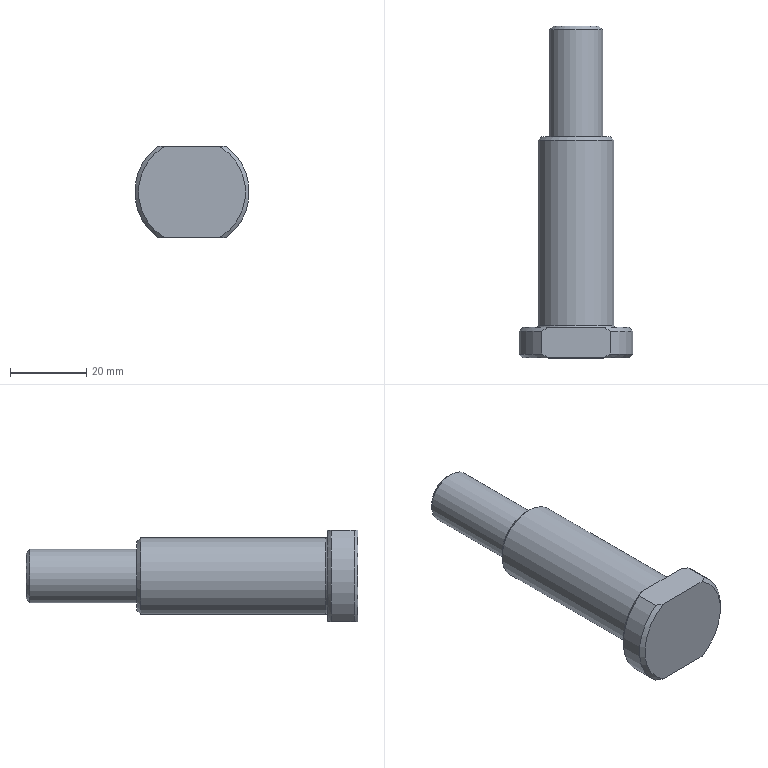Part | STEP file | HL4GZ-1.862.576 (bolt short shaft) | 1 solid | 17 faces | box 30 x 87 x 24 mm | volume 25136 mm3 | cone 6 | plane 6 | cylinder 4 | torus 1 | commonest cylinder face diameters 30 x2 14 x1 20 x1
STEP:
#1=CARTESIAN_POINT('',(0.,0.,0.));
#2=DIRECTION('',(0.,0.,1.));
#3=DIRECTION('',(1.,0.,0.));
#4=AXIS2_PLACEMENT_3D('',#1,#2,#3);
#5=CARTESIAN_POINT('',(1812.33,-148.5,34.265));
#6=VERTEX_POINT('',#5);
#7=CARTESIAN_POINT('',(1810.541,-147.5,34.265));
#8=VERTEX_POINT('',#7);
#9=CARTESIAN_POINT('',(1812.33,-148.5,34.265));
#10=CARTESIAN_POINT('',(1811.723,-148.187,34.265));
#11=CARTESIAN_POINT('',(1811.127,-147.851,34.265));
#12=CARTESIAN_POINT('',(1810.541,-147.5,34.265));
#13=B_SPLINE_CURVE_WITH_KNOTS('',3,(#9,#10,#11,#12),.UNSPECIFIED.,.F.,.F.,(4,4),(0.,1.),.PIECEWISE_BEZIER_KNOTS.);
#14=CARTESIAN_POINT('',(1819.541,-147.5,46.265));
#15=DIRECTION('',(0.,1.,0.));
#16=DIRECTION('',(0.,0.,-1.));
#17=AXIS2_PLACEMENT_3D('',#14,#15,#16);
#18=CONICAL_SURFACE('',#17,15.,0.7854);
#19=CARTESIAN_POINT('',(0.5411,-1.));
#20=CARTESIAN_POINT('',(0.6435,0.));
#21=B_SPLINE_CURVE_WITH_KNOTS('',1,(#19,#20),.UNSPECIFIED.,.F.,.F.,(2,2),(0.,1.),.PIECEWISE_BEZIER_KNOTS.);
#22=(GEOMETRIC_REPRESENTATION_CONTEXT(2)PARAMETRIC_REPRESENTATION_CONTEXT()REPRESENTATION_CONTEXT('',''));
#23=DEFINITIONAL_REPRESENTATION('',(#21),#22);
#24=PCURVE('',#18,#23);
#25=CARTESIAN_POINT('',(1831.291,-151.5,34.265));
#26=DIRECTION('',(0.,0.,1.));
#27=DIRECTION('',(-1.,0.,0.));
#28=AXIS2_PLACEMENT_3D('',#25,#26,#27);
#29=PLANE('',#28);
#30=CARTESIAN_POINT('',(18.961,-3.));
#31=CARTESIAN_POINT('',(19.568,-3.313));
#32=CARTESIAN_POINT('',(20.164,-3.649));
#33=CARTESIAN_POINT('',(20.75,-4.));
#34=B_SPLINE_CURVE_WITH_KNOTS('',3,(#30,#31,#32,#33),.UNSPECIFIED.,.F.,.F.,(4,4),(0.,1.),.PIECEWISE_BEZIER_KNOTS.);
#35=(GEOMETRIC_REPRESENTATION_CONTEXT(2)PARAMETRIC_REPRESENTATION_CONTEXT()REPRESENTATION_CONTEXT('',''));
#36=DEFINITIONAL_REPRESENTATION('',(#34),#35);
#37=PCURVE('',#29,#36);
#38=SURFACE_CURVE('',#13,(#24,#37),.PCURVE_S1.);
#39=EDGE_CURVE('',#6,#8,#38,.T.);
#40=ORIENTED_EDGE('',*,*,#39,.F.);
#41=CARTESIAN_POINT('',(1812.33,-148.5,58.265));
#42=VERTEX_POINT('',#41);
#43=CARTESIAN_POINT('',(1819.541,-148.5,46.265));
#44=DIRECTION('',(0.,-1.,0.));
#45=DIRECTION('',(0.,0.,1.));
#46=AXIS2_PLACEMENT_3D('',#43,#44,#45);
#47=CIRCLE('',#46,14.);
#48=CARTESIAN_POINT('',(3.142,-1.));
#49=DIRECTION('',(-1.,0.));
#50=VECTOR('',#49,1.);
#51=LINE('',#48,#50);
#52=(GEOMETRIC_REPRESENTATION_CONTEXT(2)PARAMETRIC_REPRESENTATION_CONTEXT()REPRESENTATION_CONTEXT('',''));
#53=DEFINITIONAL_REPRESENTATION('',(#51),#52);
#54=PCURVE('',#18,#53);
#55=CARTESIAN_POINT('',(1819.541,-148.5,46.265));
#56=DIRECTION('',(0.,1.,0.));
#57=DIRECTION('',(0.,0.,-1.));
#58=AXIS2_PLACEMENT_3D('',#55,#56,#57);
#59=PLANE('',#58);
#60=CARTESIAN_POINT('',(-14.,0.));
#61=CARTESIAN_POINT('',(-14.,24.249));
#62=CARTESIAN_POINT('',(7.,12.124));
#63=CARTESIAN_POINT('',(28.,0.));
#64=CARTESIAN_POINT('',(7.,-12.124));
#65=CARTESIAN_POINT('',(-14.,-24.249));
#66=CARTESIAN_POINT('',(-14.,0.));
#67=(BOUNDED_CURVE()B_SPLINE_CURVE(2,(#60,#61,#62,#63,#64,#65,#66),.UNSPECIFIED.,.T.,.F.)B_SPLINE_CURVE_WITH_KNOTS((1,2,2,2,2,1),(-2.094,0.,2.094,4.189,6.283,8.378),.UNSPECIFIED.)CURVE()GEOMETRIC_REPRESENTATION_ITEM()RATIONAL_B_SPLINE_CURVE((1.,0.5,1.,0.5,1.,0.5,1.))REPRESENTATION_ITEM(''));
#68=(GEOMETRIC_REPRESENTATION_CONTEXT(2)PARAMETRIC_REPRESENTATION_CONTEXT()REPRESENTATION_CONTEXT('',''));
#69=DEFINITIONAL_REPRESENTATION('',(#67),#68);
#70=PCURVE('',#59,#69);
#71=SURFACE_CURVE('',#47,(#54,#70),.PCURVE_S1.);
#72=EDGE_CURVE('',#42,#6,#71,.T.);
#73=ORIENTED_EDGE('',*,*,#72,.F.);
#74=CARTESIAN_POINT('',(1810.541,-147.5,58.265));
#75=VERTEX_POINT('',#74);
#76=CARTESIAN_POINT('',(1810.541,-147.5,58.265));
#77=CARTESIAN_POINT('',(1811.127,-147.851,58.265));
#78=CARTESIAN_POINT('',(1811.723,-148.187,58.265));
#79=CARTESIAN_POINT('',(1812.33,-148.5,58.265));
#80=B_SPLINE_CURVE_WITH_KNOTS('',3,(#76,#77,#78,#79),.UNSPECIFIED.,.F.,.F.,(4,4),(0.,1.),.PIECEWISE_BEZIER_KNOTS.);
#81=CARTESIAN_POINT('',(2.498,0.));
#82=CARTESIAN_POINT('',(2.6,-1.));
#83=B_SPLINE_CURVE_WITH_KNOTS('',1,(#81,#82),.UNSPECIFIED.,.F.,.F.,(2,2),(0.,1.),.PIECEWISE_BEZIER_KNOTS.);
#84=(GEOMETRIC_REPRESENTATION_CONTEXT(2)PARAMETRIC_REPRESENTATION_CONTEXT()REPRESENTATION_CONTEXT('',''));
#85=DEFINITIONAL_REPRESENTATION('',(#83),#84);
#86=PCURVE('',#18,#85);
#87=CARTESIAN_POINT('',(1835.541,-151.5,58.265));
#88=DIRECTION('',(0.,0.,-1.));
#89=DIRECTION('',(1.,0.,0.));
#90=AXIS2_PLACEMENT_3D('',#87,#88,#89);
#91=PLANE('',#90);
#92=CARTESIAN_POINT('',(-25.,-4.));
#93=CARTESIAN_POINT('',(-24.414,-3.649));
#94=CARTESIAN_POINT('',(-23.818,-3.313));
#95=CARTESIAN_POINT('',(-23.211,-3.));
#96=B_SPLINE_CURVE_WITH_KNOTS('',3,(#92,#93,#94,#95),.UNSPECIFIED.,.F.,.F.,(4,4),(0.,1.),.PIECEWISE_BEZIER_KNOTS.);
#97=(GEOMETRIC_REPRESENTATION_CONTEXT(2)PARAMETRIC_REPRESENTATION_CONTEXT()REPRESENTATION_CONTEXT('',''));
#98=DEFINITIONAL_REPRESENTATION('',(#96),#97);
#99=PCURVE('',#91,#98);
#100=SURFACE_CURVE('',#80,(#86,#99),.PCURVE_S1.);
#101=EDGE_CURVE('',#75,#42,#100,.T.);
#102=ORIENTED_EDGE('',*,*,#101,.F.);
#103=CARTESIAN_POINT('',(1819.541,-147.5,46.265));
#104=DIRECTION('',(0.,1.,0.));
#105=DIRECTION('',(0.,0.,1.));
#106=AXIS2_PLACEMENT_3D('',#103,#104,#105);
#107=CIRCLE('',#106,15.);
#108=CARTESIAN_POINT('',(-3.142,0.));
#109=DIRECTION('',(1.,0.));
#110=VECTOR('',#109,1.);
#111=LINE('',#108,#110);
#112=(GEOMETRIC_REPRESENTATION_CONTEXT(2)PARAMETRIC_REPRESENTATION_CONTEXT()REPRESENTATION_CONTEXT('',''));
#113=DEFINITIONAL_REPRESENTATION('',(#111),#112);
#114=PCURVE('',#18,#113);
#115=CARTESIAN_POINT('',(1819.541,-140.5,46.265));
#116=DIRECTION('',(0.,1.,0.));
#117=DIRECTION('',(0.,0.,-1.));
#118=AXIS2_PLACEMENT_3D('',#115,#116,#117);
#119=CYLINDRICAL_SURFACE('',#118,15.);
#120=CARTESIAN_POINT('',(-3.142,-7.));
#121=DIRECTION('',(1.,0.));
#122=VECTOR('',#121,1.);
#123=LINE('',#120,#122);
#124=(GEOMETRIC_REPRESENTATION_CONTEXT(2)PARAMETRIC_REPRESENTATION_CONTEXT()REPRESENTATION_CONTEXT('',''));
#125=DEFINITIONAL_REPRESENTATION('',(#123),#124);
#126=PCURVE('',#119,#125);
#127=SURFACE_CURVE('',#107,(#114,#126),.PCURVE_S1.);
#128=EDGE_CURVE('',#8,#75,#127,.T.);
#129=ORIENTED_EDGE('',*,*,#128,.F.);
#130=EDGE_LOOP('',(#40,#73,#102,#129));
#131=FACE_BOUND('',#130,.T.);
#132=ADVANCED_FACE('',(#131),#18,.T.);
#133=CARTESIAN_POINT('',(1810.541,-141.5,34.265));
#134=VERTEX_POINT('',#133);
#135=CARTESIAN_POINT('',(1812.33,-140.5,34.265));
#136=VERTEX_POINT('',#135);
#137=CARTESIAN_POINT('',(1810.541,-141.5,34.265));
#138=CARTESIAN_POINT('',(1811.127,-141.148,34.265));
#139=CARTESIAN_POINT('',(1811.723,-140.813,34.265));
#140=CARTESIAN_POINT('',(1812.33,-140.5,34.265));
#141=B_SPLINE_CURVE_WITH_KNOTS('',3,(#137,#138,#139,#140),.UNSPECIFIED.,.F.,.F.,(4,4),(0.,1.),.PIECEWISE_BEZIER_KNOTS.);
#142=CARTESIAN_POINT('',(1819.541,-140.5,46.265));
#143=DIRECTION('',(0.,-1.,0.));
#144=DIRECTION('',(0.,0.,1.));
#145=AXIS2_PLACEMENT_3D('',#142,#143,#144);
#146=CONICAL_SURFACE('',#145,14.,0.7854);
#147=CARTESIAN_POINT('',(2.498,1.));
#148=CARTESIAN_POINT('',(2.6,0.));
#149=B_SPLINE_CURVE_WITH_KNOTS('',1,(#147,#148),.UNSPECIFIED.,.F.,.F.,(2,2),(0.,1.),.PIECEWISE_BEZIER_KNOTS.);
#150=(GEOMETRIC_REPRESENTATION_CONTEXT(2)PARAMETRIC_REPRESENTATION_CONTEXT()REPRESENTATION_CONTEXT('',''));
#151=DEFINITIONAL_REPRESENTATION('',(#149),#150);
#152=PCURVE('',#146,#151);
#153=CARTESIAN_POINT('',(20.75,-10.));
#154=CARTESIAN_POINT('',(20.164,-10.351));
#155=CARTESIAN_POINT('',(19.568,-10.687));
#156=CARTESIAN_POINT('',(18.961,-11.));
#157=B_SPLINE_CURVE_WITH_KNOTS('',3,(#153,#154,#155,#156),.UNSPECIFIED.,.F.,.F.,(4,4),(0.,1.),.PIECEWISE_BEZIER_KNOTS.);
#158=(GEOMETRIC_REPRESENTATION_CONTEXT(2)PARAMETRIC_REPRESENTATION_CONTEXT()REPRESENTATION_CONTEXT('',''));
#159=DEFINITIONAL_REPRESENTATION('',(#157),#158);
#160=PCURVE('',#29,#159);
#161=SURFACE_CURVE('',#141,(#152,#160),.PCURVE_S1.);
#162=EDGE_CURVE('',#134,#136,#161,.T.);
#163=ORIENTED_EDGE('',*,*,#162,.F.);
#164=CARTESIAN_POINT('',(1810.541,-141.5,58.265));
#165=VERTEX_POINT('',#164);
#166=CARTESIAN_POINT('',(1819.541,-141.5,46.265));
#167=DIRECTION('',(0.,-1.,0.));
#168=DIRECTION('',(0.,0.,1.));
#169=AXIS2_PLACEMENT_3D('',#166,#167,#168);
#170=CIRCLE('',#169,15.);
#171=CARTESIAN_POINT('',(0.,1.));
#172=DIRECTION('',(1.,0.));
#173=VECTOR('',#172,1.);
#174=LINE('',#171,#173);
#175=(GEOMETRIC_REPRESENTATION_CONTEXT(2)PARAMETRIC_REPRESENTATION_CONTEXT()REPRESENTATION_CONTEXT('',''));
#176=DEFINITIONAL_REPRESENTATION('',(#174),#175);
#177=PCURVE('',#146,#176);
#178=CARTESIAN_POINT('',(3.142,-1.));
#179=DIRECTION('',(-1.,0.));
#180=VECTOR('',#179,1.);
#181=LINE('',#178,#180);
#182=(GEOMETRIC_REPRESENTATION_CONTEXT(2)PARAMETRIC_REPRESENTATION_CONTEXT()REPRESENTATION_CONTEXT('',''));
#183=DEFINITIONAL_REPRESENTATION('',(#181),#182);
#184=PCURVE('',#119,#183);
#185=SURFACE_CURVE('',#170,(#177,#184),.PCURVE_S1.);
#186=EDGE_CURVE('',#165,#134,#185,.T.);
#187=ORIENTED_EDGE('',*,*,#186,.F.);
#188=CARTESIAN_POINT('',(1812.33,-140.5,58.265));
#189=VERTEX_POINT('',#188);
#190=CARTESIAN_POINT('',(1812.33,-140.5,58.265));
#191=CARTESIAN_POINT('',(1811.723,-140.813,58.265));
#192=CARTESIAN_POINT('',(1811.127,-141.148,58.265));
#193=CARTESIAN_POINT('',(1810.541,-141.5,58.265));
#194=B_SPLINE_CURVE_WITH_KNOTS('',3,(#190,#191,#192,#193),.UNSPECIFIED.,.F.,.F.,(4,4),(0.,1.),.PIECEWISE_BEZIER_KNOTS.);
#195=CARTESIAN_POINT('',(0.5411,0.));
#196=CARTESIAN_POINT('',(0.6435,1.));
#197=B_SPLINE_CURVE_WITH_KNOTS('',1,(#195,#196),.UNSPECIFIED.,.F.,.F.,(2,2),(0.,1.),.PIECEWISE_BEZIER_KNOTS.);
#198=(GEOMETRIC_REPRESENTATION_CONTEXT(2)PARAMETRIC_REPRESENTATION_CONTEXT()REPRESENTATION_CONTEXT('',''));
#199=DEFINITIONAL_REPRESENTATION('',(#197),#198);
#200=PCURVE('',#146,#199);
#201=CARTESIAN_POINT('',(-23.211,-11.));
#202=CARTESIAN_POINT('',(-23.818,-10.687));
#203=CARTESIAN_POINT('',(-24.414,-10.351));
#204=CARTESIAN_POINT('',(-25.,-10.));
#205=B_SPLINE_CURVE_WITH_KNOTS('',3,(#201,#202,#203,#204),.UNSPECIFIED.,.F.,.F.,(4,4),(0.,1.),.PIECEWISE_BEZIER_KNOTS.);
#206=(GEOMETRIC_REPRESENTATION_CONTEXT(2)PARAMETRIC_REPRESENTATION_CONTEXT()REPRESENTATION_CONTEXT('',''));
#207=DEFINITIONAL_REPRESENTATION('',(#205),#206);
#208=PCURVE('',#91,#207);
#209=SURFACE_CURVE('',#194,(#200,#208),.PCURVE_S1.);
#210=EDGE_CURVE('',#189,#165,#209,.T.);
#211=ORIENTED_EDGE('',*,*,#210,.F.);
#212=CARTESIAN_POINT('',(1819.541,-140.5,46.265));
#213=DIRECTION('',(0.,1.,0.));
#214=DIRECTION('',(0.,0.,1.));
#215=AXIS2_PLACEMENT_3D('',#212,#213,#214);
#216=CIRCLE('',#215,14.);
#217=CARTESIAN_POINT('',(6.283,0.));
#218=DIRECTION('',(-1.,0.));
#219=VECTOR('',#218,1.);
#220=LINE('',#217,#219);
#221=(GEOMETRIC_REPRESENTATION_CONTEXT(2)PARAMETRIC_REPRESENTATION_CONTEXT()REPRESENTATION_CONTEXT('',''));
#222=DEFINITIONAL_REPRESENTATION('',(#220),#221);
#223=PCURVE('',#146,#222);
#224=CARTESIAN_POINT('',(1804.541,-140.5,46.265));
#225=DIRECTION('',(0.,1.,0.));
#226=DIRECTION('',(0.,0.,-1.));
#227=AXIS2_PLACEMENT_3D('',#224,#225,#226);
#228=PLANE('',#227);
#229=CARTESIAN_POINT('',(0.,-15.));
#230=DIRECTION('',(-1.,0.));
#231=AXIS2_PLACEMENT_2D('',#229,#230);
#232=CIRCLE('',#231,14.);
#233=(GEOMETRIC_REPRESENTATION_CONTEXT(2)PARAMETRIC_REPRESENTATION_CONTEXT()REPRESENTATION_CONTEXT('',''));
#234=DEFINITIONAL_REPRESENTATION('',(#232),#233);
#235=PCURVE('',#228,#234);
#236=SURFACE_CURVE('',#216,(#223,#235),.PCURVE_S1.);
#237=EDGE_CURVE('',#136,#189,#236,.T.);
#238=ORIENTED_EDGE('',*,*,#237,.F.);
#239=EDGE_LOOP('',(#163,#187,#211,#238));
#240=FACE_BOUND('',#239,.T.);
#241=ADVANCED_FACE('',(#240),#146,.T.);
#242=CARTESIAN_POINT('',(1828.541,-141.5,58.265));
#243=VERTEX_POINT('',#242);
#244=CARTESIAN_POINT('',(1826.752,-140.5,58.265));
#245=VERTEX_POINT('',#244);
#246=CARTESIAN_POINT('',(1828.541,-141.5,58.265));
#247=CARTESIAN_POINT('',(1827.955,-141.148,58.265));
#248=CARTESIAN_POINT('',(1827.36,-140.813,58.265));
#249=CARTESIAN_POINT('',(1826.752,-140.5,58.265));
#250=B_SPLINE_CURVE_WITH_KNOTS('',3,(#246,#247,#248,#249),.UNSPECIFIED.,.F.,.F.,(4,4),(0.,1.),.PIECEWISE_BEZIER_KNOTS.);
#251=CARTESIAN_POINT('',(1819.541,-140.5,46.265));
#252=DIRECTION('',(0.,-1.,0.));
#253=DIRECTION('',(0.,0.,1.));
#254=AXIS2_PLACEMENT_3D('',#251,#252,#253);
#255=CONICAL_SURFACE('',#254,14.,0.7854);
#256=CARTESIAN_POINT('',(5.64,1.));
#257=CARTESIAN_POINT('',(5.742,0.));
#258=B_SPLINE_CURVE_WITH_KNOTS('',1,(#256,#257),.UNSPECIFIED.,.F.,.F.,(2,2),(0.,1.),.PIECEWISE_BEZIER_KNOTS.);
#259=(GEOMETRIC_REPRESENTATION_CONTEXT(2)PARAMETRIC_REPRESENTATION_CONTEXT()REPRESENTATION_CONTEXT('',''));
#260=DEFINITIONAL_REPRESENTATION('',(#258),#259);
#261=PCURVE('',#255,#260);
#262=CARTESIAN_POINT('',(-7.,-10.));
#263=CARTESIAN_POINT('',(-7.586,-10.351));
#264=CARTESIAN_POINT('',(-8.182,-10.687));
#265=CARTESIAN_POINT('',(-8.789,-11.));
#266=B_SPLINE_CURVE_WITH_KNOTS('',3,(#262,#263,#264,#265),.UNSPECIFIED.,.F.,.F.,(4,4),(0.,1.),.PIECEWISE_BEZIER_KNOTS.);
#267=(GEOMETRIC_REPRESENTATION_CONTEXT(2)PARAMETRIC_REPRESENTATION_CONTEXT()REPRESENTATION_CONTEXT('',''));
#268=DEFINITIONAL_REPRESENTATION('',(#266),#267);
#269=PCURVE('',#91,#268);
#270=SURFACE_CURVE('',#250,(#261,#269),.PCURVE_S1.);
#271=EDGE_CURVE('',#243,#245,#270,.T.);
#272=ORIENTED_EDGE('',*,*,#271,.F.);
#273=CARTESIAN_POINT('',(1828.541,-141.5,34.265));
#274=VERTEX_POINT('',#273);
#275=CARTESIAN_POINT('',(1819.541,-141.5,46.265));
#276=DIRECTION('',(0.,-1.,0.));
#277=DIRECTION('',(0.,0.,1.));
#278=AXIS2_PLACEMENT_3D('',#275,#276,#277);
#279=CIRCLE('',#278,15.);
#280=CARTESIAN_POINT('',(0.,1.));
#281=DIRECTION('',(1.,0.));
#282=VECTOR('',#281,1.);
#283=LINE('',#280,#282);
#284=(GEOMETRIC_REPRESENTATION_CONTEXT(2)PARAMETRIC_REPRESENTATION_CONTEXT()REPRESENTATION_CONTEXT('',''));
#285=DEFINITIONAL_REPRESENTATION('',(#283),#284);
#286=PCURVE('',#255,#285);
#287=CARTESIAN_POINT('',(1819.541,-140.5,46.265));
#288=DIRECTION('',(0.,1.,0.));
#289=DIRECTION('',(0.,0.,-1.));
#290=AXIS2_PLACEMENT_3D('',#287,#288,#289);
#291=CYLINDRICAL_SURFACE('',#290,15.);
#292=CARTESIAN_POINT('',(9.425,-1.));
#293=DIRECTION('',(-1.,0.));
#294=VECTOR('',#293,1.);
#295=LINE('',#292,#294);
#296=(GEOMETRIC_REPRESENTATION_CONTEXT(2)PARAMETRIC_REPRESENTATION_CONTEXT()REPRESENTATION_CONTEXT('',''));
#297=DEFINITIONAL_REPRESENTATION('',(#295),#296);
#298=PCURVE('',#291,#297);
#299=SURFACE_CURVE('',#279,(#286,#298),.PCURVE_S1.);
#300=EDGE_CURVE('',#274,#243,#299,.T.);
#301=ORIENTED_EDGE('',*,*,#300,.F.);
#302=CARTESIAN_POINT('',(1826.752,-140.5,34.265));
#303=VERTEX_POINT('',#302);
#304=CARTESIAN_POINT('',(1826.752,-140.5,34.265));
#305=CARTESIAN_POINT('',(1827.36,-140.813,34.265));
#306=CARTESIAN_POINT('',(1827.955,-141.148,34.265));
#307=CARTESIAN_POINT('',(1828.541,-141.5,34.265));
#308=B_SPLINE_CURVE_WITH_KNOTS('',3,(#304,#305,#306,#307),.UNSPECIFIED.,.F.,.F.,(4,4),(0.,1.),.PIECEWISE_BEZIER_KNOTS.);
#309=CARTESIAN_POINT('',(3.683,0.));
#310=CARTESIAN_POINT('',(3.785,1.));
#311=B_SPLINE_CURVE_WITH_KNOTS('',1,(#309,#310),.UNSPECIFIED.,.F.,.F.,(2,2),(0.,1.),.PIECEWISE_BEZIER_KNOTS.);
#312=(GEOMETRIC_REPRESENTATION_CONTEXT(2)PARAMETRIC_REPRESENTATION_CONTEXT()REPRESENTATION_CONTEXT('',''));
#313=DEFINITIONAL_REPRESENTATION('',(#311),#312);
#314=PCURVE('',#255,#313);
#315=CARTESIAN_POINT('',(4.539,-11.));
#316=CARTESIAN_POINT('',(3.932,-10.687));
#317=CARTESIAN_POINT('',(3.336,-10.351));
#318=CARTESIAN_POINT('',(2.75,-10.));
#319=B_SPLINE_CURVE_WITH_KNOTS('',3,(#315,#316,#317,#318),.UNSPECIFIED.,.F.,.F.,(4,4),(0.,1.),.PIECEWISE_BEZIER_KNOTS.);
#320=(GEOMETRIC_REPRESENTATION_CONTEXT(2)PARAMETRIC_REPRESENTATION_CONTEXT()REPRESENTATION_CONTEXT('',''));
#321=DEFINITIONAL_REPRESENTATION('',(#319),#320);
#322=PCURVE('',#29,#321);
#323=SURFACE_CURVE('',#308,(#314,#322),.PCURVE_S1.);
#324=EDGE_CURVE('',#303,#274,#323,.T.);
#325=ORIENTED_EDGE('',*,*,#324,.F.);
#326=CARTESIAN_POINT('',(1819.541,-140.5,46.265));
#327=DIRECTION('',(0.,1.,0.));
#328=DIRECTION('',(0.,0.,1.));
#329=AXIS2_PLACEMENT_3D('',#326,#327,#328);
#330=CIRCLE('',#329,14.);
#331=CARTESIAN_POINT('',(6.283,0.));
#332=DIRECTION('',(-1.,0.));
#333=VECTOR('',#332,1.);
#334=LINE('',#331,#333);
#335=(GEOMETRIC_REPRESENTATION_CONTEXT(2)PARAMETRIC_REPRESENTATION_CONTEXT()REPRESENTATION_CONTEXT('',''));
#336=DEFINITIONAL_REPRESENTATION('',(#334),#335);
#337=PCURVE('',#255,#336);
#338=CARTESIAN_POINT('',(0.,-15.));
#339=DIRECTION('',(-1.,0.));
#340=AXIS2_PLACEMENT_2D('',#338,#339);
#341=CIRCLE('',#340,14.);
#342=(GEOMETRIC_REPRESENTATION_CONTEXT(2)PARAMETRIC_REPRESENTATION_CONTEXT()REPRESENTATION_CONTEXT('',''));
#343=DEFINITIONAL_REPRESENTATION('',(#341),#342);
#344=PCURVE('',#228,#343);
#345=SURFACE_CURVE('',#330,(#337,#344),.PCURVE_S1.);
#346=EDGE_CURVE('',#245,#303,#345,.T.);
#347=ORIENTED_EDGE('',*,*,#346,.F.);
#348=EDGE_LOOP('',(#272,#301,#325,#347));
#349=FACE_BOUND('',#348,.T.);
#350=ADVANCED_FACE('',(#349),#255,.T.);
#351=CARTESIAN_POINT('',(1826.752,-148.5,58.265));
#352=VERTEX_POINT('',#351);
#353=CARTESIAN_POINT('',(1828.541,-147.5,58.265));
#354=VERTEX_POINT('',#353);
#355=CARTESIAN_POINT('',(1826.752,-148.5,58.265));
#356=CARTESIAN_POINT('',(1827.36,-148.187,58.265));
#357=CARTESIAN_POINT('',(1827.955,-147.851,58.265));
#358=CARTESIAN_POINT('',(1828.541,-147.5,58.265));
#359=B_SPLINE_CURVE_WITH_KNOTS('',3,(#355,#356,#357,#358),.UNSPECIFIED.,.F.,.F.,(4,4),(0.,1.),.PIECEWISE_BEZIER_KNOTS.);
#360=CARTESIAN_POINT('',(1819.541,-147.5,46.265));
#361=DIRECTION('',(0.,1.,0.));
#362=DIRECTION('',(0.,0.,-1.));
#363=AXIS2_PLACEMENT_3D('',#360,#361,#362);
#364=CONICAL_SURFACE('',#363,15.,0.7854);
#365=CARTESIAN_POINT('',(3.683,-1.));
#366=CARTESIAN_POINT('',(3.785,0.));
#367=B_SPLINE_CURVE_WITH_KNOTS('',1,(#365,#366),.UNSPECIFIED.,.F.,.F.,(2,2),(0.,1.),.PIECEWISE_BEZIER_KNOTS.);
#368=(GEOMETRIC_REPRESENTATION_CONTEXT(2)PARAMETRIC_REPRESENTATION_CONTEXT()REPRESENTATION_CONTEXT('',''));
#369=DEFINITIONAL_REPRESENTATION('',(#367),#368);
#370=PCURVE('',#364,#369);
#371=CARTESIAN_POINT('',(-8.789,-3.));
#372=CARTESIAN_POINT('',(-8.182,-3.313));
#373=CARTESIAN_POINT('',(-7.586,-3.649));
#374=CARTESIAN_POINT('',(-7.,-4.));
#375=B_SPLINE_CURVE_WITH_KNOTS('',3,(#371,#372,#373,#374),.UNSPECIFIED.,.F.,.F.,(4,4),(0.,1.),.PIECEWISE_BEZIER_KNOTS.);
#376=(GEOMETRIC_REPRESENTATION_CONTEXT(2)PARAMETRIC_REPRESENTATION_CONTEXT()REPRESENTATION_CONTEXT('',''));
#377=DEFINITIONAL_REPRESENTATION('',(#375),#376);
#378=PCURVE('',#91,#377);
#379=SURFACE_CURVE('',#359,(#370,#378),.PCURVE_S1.);
#380=EDGE_CURVE('',#352,#354,#379,.T.);
#381=ORIENTED_EDGE('',*,*,#380,.F.);
#382=CARTESIAN_POINT('',(1826.752,-148.5,34.265));
#383=VERTEX_POINT('',#382);
#384=CARTESIAN_POINT('',(1819.541,-148.5,46.265));
#385=DIRECTION('',(0.,-1.,0.));
#386=DIRECTION('',(0.,0.,1.));
#387=AXIS2_PLACEMENT_3D('',#384,#385,#386);
#388=CIRCLE('',#387,14.);
#389=CARTESIAN_POINT('',(9.425,-1.));
#390=DIRECTION('',(-1.,0.));
#391=VECTOR('',#390,1.);
#392=LINE('',#389,#391);
#393=(GEOMETRIC_REPRESENTATION_CONTEXT(2)PARAMETRIC_REPRESENTATION_CONTEXT()REPRESENTATION_CONTEXT('',''));
#394=DEFINITIONAL_REPRESENTATION('',(#392),#393);
#395=PCURVE('',#364,#394);
#396=CARTESIAN_POINT('',(-14.,0.));
#397=CARTESIAN_POINT('',(-14.,24.249));
#398=CARTESIAN_POINT('',(7.,12.124));
#399=CARTESIAN_POINT('',(28.,0.));
#400=CARTESIAN_POINT('',(7.,-12.124));
#401=CARTESIAN_POINT('',(-14.,-24.249));
#402=CARTESIAN_POINT('',(-14.,0.));
#403=(BOUNDED_CURVE()B_SPLINE_CURVE(2,(#396,#397,#398,#399,#400,#401,#402),.UNSPECIFIED.,.T.,.F.)B_SPLINE_CURVE_WITH_KNOTS((1,2,2,2,2,1),(-2.094,0.,2.094,4.189,6.283,8.378),.UNSPECIFIED.)CURVE()GEOMETRIC_REPRESENTATION_ITEM()RATIONAL_B_SPLINE_CURVE((1.,0.5,1.,0.5,1.,0.5,1.))REPRESENTATION_ITEM(''));
#404=(GEOMETRIC_REPRESENTATION_CONTEXT(2)PARAMETRIC_REPRESENTATION_CONTEXT()REPRESENTATION_CONTEXT('',''));
#405=DEFINITIONAL_REPRESENTATION('',(#403),#404);
#406=PCURVE('',#59,#405);
#407=SURFACE_CURVE('',#388,(#395,#406),.PCURVE_S1.);
#408=EDGE_CURVE('',#383,#352,#407,.T.);
#409=ORIENTED_EDGE('',*,*,#408,.F.);
#410=CARTESIAN_POINT('',(1828.541,-147.5,34.265));
#411=VERTEX_POINT('',#410);
#412=CARTESIAN_POINT('',(1828.541,-147.5,34.265));
#413=CARTESIAN_POINT('',(1827.955,-147.851,34.265));
#414=CARTESIAN_POINT('',(1827.36,-148.187,34.265));
#415=CARTESIAN_POINT('',(1826.752,-148.5,34.265));
#416=B_SPLINE_CURVE_WITH_KNOTS('',3,(#412,#413,#414,#415),.UNSPECIFIED.,.F.,.F.,(4,4),(0.,1.),.PIECEWISE_BEZIER_KNOTS.);
#417=CARTESIAN_POINT('',(5.64,0.));
#418=CARTESIAN_POINT('',(5.742,-1.));
#419=B_SPLINE_CURVE_WITH_KNOTS('',1,(#417,#418),.UNSPECIFIED.,.F.,.F.,(2,2),(0.,1.),.PIECEWISE_BEZIER_KNOTS.);
#420=(GEOMETRIC_REPRESENTATION_CONTEXT(2)PARAMETRIC_REPRESENTATION_CONTEXT()REPRESENTATION_CONTEXT('',''));
#421=DEFINITIONAL_REPRESENTATION('',(#419),#420);
#422=PCURVE('',#364,#421);
#423=CARTESIAN_POINT('',(2.75,-4.));
#424=CARTESIAN_POINT('',(3.336,-3.649));
#425=CARTESIAN_POINT('',(3.932,-3.313));
#426=CARTESIAN_POINT('',(4.539,-3.));
#427=B_SPLINE_CURVE_WITH_KNOTS('',3,(#423,#424,#425,#426),.UNSPECIFIED.,.F.,.F.,(4,4),(0.,1.),.PIECEWISE_BEZIER_KNOTS.);
#428=(GEOMETRIC_REPRESENTATION_CONTEXT(2)PARAMETRIC_REPRESENTATION_CONTEXT()REPRESENTATION_CONTEXT('',''));
#429=DEFINITIONAL_REPRESENTATION('',(#427),#428);
#430=PCURVE('',#29,#429);
#431=SURFACE_CURVE('',#416,(#422,#430),.PCURVE_S1.);
#432=EDGE_CURVE('',#411,#383,#431,.T.);
#433=ORIENTED_EDGE('',*,*,#432,.F.);
#434=CARTESIAN_POINT('',(1819.541,-147.5,46.265));
#435=DIRECTION('',(0.,1.,0.));
#436=DIRECTION('',(0.,0.,1.));
#437=AXIS2_PLACEMENT_3D('',#434,#435,#436);
#438=CIRCLE('',#437,15.);
#439=CARTESIAN_POINT('',(3.142,0.));
#440=DIRECTION('',(1.,0.));
#441=VECTOR('',#440,1.);
#442=LINE('',#439,#441);
#443=(GEOMETRIC_REPRESENTATION_CONTEXT(2)PARAMETRIC_REPRESENTATION_CONTEXT()REPRESENTATION_CONTEXT('',''));
#444=DEFINITIONAL_REPRESENTATION('',(#442),#443);
#445=PCURVE('',#364,#444);
#446=CARTESIAN_POINT('',(3.142,-7.));
#447=DIRECTION('',(1.,0.));
#448=VECTOR('',#447,1.);
#449=LINE('',#446,#448);
#450=(GEOMETRIC_REPRESENTATION_CONTEXT(2)PARAMETRIC_REPRESENTATION_CONTEXT()REPRESENTATION_CONTEXT('',''));
#451=DEFINITIONAL_REPRESENTATION('',(#449),#450);
#452=PCURVE('',#291,#451);
#453=SURFACE_CURVE('',#438,(#445,#452),.PCURVE_S1.);
#454=EDGE_CURVE('',#354,#411,#453,.T.);
#455=ORIENTED_EDGE('',*,*,#454,.F.);
#456=EDGE_LOOP('',(#381,#409,#433,#455));
#457=FACE_BOUND('',#456,.T.);
#458=ADVANCED_FACE('',(#457),#364,.T.);
#459=CARTESIAN_POINT('',(1819.541,-91.5,56.265));
#460=VERTEX_POINT('',#459);
#461=CARTESIAN_POINT('',(1819.541,-91.5,46.265));
#462=DIRECTION('',(0.,-1.,0.));
#463=DIRECTION('',(0.,0.,1.));
#464=AXIS2_PLACEMENT_3D('',#461,#462,#463);
#465=CIRCLE('',#464,10.);
#466=CARTESIAN_POINT('',(1819.541,-91.5,46.265));
#467=DIRECTION('',(0.,-1.,0.));
#468=DIRECTION('',(0.,0.,1.));
#469=AXIS2_PLACEMENT_3D('',#466,#467,#468);
#470=CONICAL_SURFACE('',#469,10.,0.7854);
#471=CARTESIAN_POINT('',(0.,0.));
#472=DIRECTION('',(1.,0.));
#473=VECTOR('',#472,1.);
#474=LINE('',#471,#473);
#475=(GEOMETRIC_REPRESENTATION_CONTEXT(2)PARAMETRIC_REPRESENTATION_CONTEXT()REPRESENTATION_CONTEXT('',''));
#476=DEFINITIONAL_REPRESENTATION('',(#474),#475);
#477=PCURVE('',#470,#476);
#478=CARTESIAN_POINT('',(1819.541,-140.5,46.265));
#479=DIRECTION('',(0.,1.,0.));
#480=DIRECTION('',(0.,0.,-1.));
#481=AXIS2_PLACEMENT_3D('',#478,#479,#480);
#482=CYLINDRICAL_SURFACE('',#481,10.);
#483=CARTESIAN_POINT('',(9.425,49.));
#484=DIRECTION('',(-1.,0.));
#485=VECTOR('',#484,1.);
#486=LINE('',#483,#485);
#487=(GEOMETRIC_REPRESENTATION_CONTEXT(2)PARAMETRIC_REPRESENTATION_CONTEXT()REPRESENTATION_CONTEXT('',''));
#488=DEFINITIONAL_REPRESENTATION('',(#486),#487);
#489=PCURVE('',#482,#488);
#490=SURFACE_CURVE('',#465,(#477,#489),.PCURVE_S1.);
#491=EDGE_CURVE('',#460,#460,#490,.T.);
#492=ORIENTED_EDGE('',*,*,#491,.F.);
#493=CARTESIAN_POINT('',(1819.541,-90.5,55.265));
#494=VERTEX_POINT('',#493);
#495=CARTESIAN_POINT('',(1819.541,-90.5,55.265));
#496=CARTESIAN_POINT('',(1819.541,-91.5,56.265));
#497=B_SPLINE_CURVE_WITH_KNOTS('',1,(#495,#496),.UNSPECIFIED.,.F.,.F.,(2,2),(-1.414,0.),.PIECEWISE_BEZIER_KNOTS.);
#498=CARTESIAN_POINT('',(0.,0.));
#499=DIRECTION('',(0.,1.));
#500=VECTOR('',#499,1.);
#501=LINE('',#498,#500);
#502=(GEOMETRIC_REPRESENTATION_CONTEXT(2)PARAMETRIC_REPRESENTATION_CONTEXT()REPRESENTATION_CONTEXT('',''));
#503=DEFINITIONAL_REPRESENTATION('',(#501),#502);
#504=PCURVE('',#470,#503);
#505=CARTESIAN_POINT('',(6.283,0.));
#506=DIRECTION('',(0.,1.));
#507=VECTOR('',#506,1.);
#508=LINE('',#505,#507);
#509=(GEOMETRIC_REPRESENTATION_CONTEXT(2)PARAMETRIC_REPRESENTATION_CONTEXT()REPRESENTATION_CONTEXT('',''));
#510=DEFINITIONAL_REPRESENTATION('',(#508),#509);
#511=PCURVE('',#470,#510);
#512=SEAM_CURVE('',#497,(#504,#511),.PCURVE_S1.);
#513=EDGE_CURVE('',#494,#460,#512,.T.);
#514=ORIENTED_EDGE('',*,*,#513,.F.);
#515=CARTESIAN_POINT('',(1819.541,-90.5,46.265));
#516=DIRECTION('',(0.,1.,0.));
#517=DIRECTION('',(0.,0.,1.));
#518=AXIS2_PLACEMENT_3D('',#515,#516,#517);
#519=CIRCLE('',#518,9.);
#520=CARTESIAN_POINT('',(6.283,-1.));
#521=DIRECTION('',(-1.,0.));
#522=VECTOR('',#521,1.);
#523=LINE('',#520,#522);
#524=(GEOMETRIC_REPRESENTATION_CONTEXT(2)PARAMETRIC_REPRESENTATION_CONTEXT()REPRESENTATION_CONTEXT('',''));
#525=DEFINITIONAL_REPRESENTATION('',(#523),#524);
#526=PCURVE('',#470,#525);
#527=CARTESIAN_POINT('',(1809.541,-90.5,46.265));
#528=DIRECTION('',(0.,1.,0.));
#529=DIRECTION('',(0.,0.,-1.));
#530=AXIS2_PLACEMENT_3D('',#527,#528,#529);
#531=PLANE('',#530);
#532=CARTESIAN_POINT('',(0.,-10.));
#533=DIRECTION('',(-1.,0.));
#534=AXIS2_PLACEMENT_2D('',#532,#533);
#535=CIRCLE('',#534,9.);
#536=(GEOMETRIC_REPRESENTATION_CONTEXT(2)PARAMETRIC_REPRESENTATION_CONTEXT()REPRESENTATION_CONTEXT('',''));
#537=DEFINITIONAL_REPRESENTATION('',(#535),#536);
#538=PCURVE('',#531,#537);
#539=SURFACE_CURVE('',#519,(#526,#538),.PCURVE_S1.);
#540=EDGE_CURVE('',#494,#494,#539,.T.);
#541=ORIENTED_EDGE('',*,*,#540,.F.);
#542=ORIENTED_EDGE('',*,*,#513,.T.);
#543=EDGE_LOOP('',(#492,#514,#541,#542));
#544=FACE_BOUND('',#543,.T.);
#545=ADVANCED_FACE('',(#544),#470,.T.);
#546=CARTESIAN_POINT('',(1819.541,-140.,56.265));
#547=VERTEX_POINT('',#546);
#548=CARTESIAN_POINT('',(1819.541,-140.,46.265));
#549=DIRECTION('',(0.,1.,0.));
#550=DIRECTION('',(0.,0.,1.));
#551=AXIS2_PLACEMENT_3D('',#548,#549,#550);
#552=CIRCLE('',#551,10.);
#553=CARTESIAN_POINT('',(1819.541,-140.,46.265));
#554=DIRECTION('',(0.,1.,0.));
#555=DIRECTION('',(0.,0.,-1.));
#556=AXIS2_PLACEMENT_3D('',#553,#554,#555);
#557=TOROIDAL_SURFACE('',#556,10.5,0.5);
#558=CARTESIAN_POINT('',(3.142,3.142));
#559=DIRECTION('',(1.,0.));
#560=VECTOR('',#559,1.);
#561=LINE('',#558,#560);
#562=(GEOMETRIC_REPRESENTATION_CONTEXT(2)PARAMETRIC_REPRESENTATION_CONTEXT()REPRESENTATION_CONTEXT('',''));
#563=DEFINITIONAL_REPRESENTATION('',(#561),#562);
#564=PCURVE('',#557,#563);
#565=CARTESIAN_POINT('',(3.142,0.5));
#566=DIRECTION('',(1.,0.));
#567=VECTOR('',#566,1.);
#568=LINE('',#565,#567);
#569=(GEOMETRIC_REPRESENTATION_CONTEXT(2)PARAMETRIC_REPRESENTATION_CONTEXT()REPRESENTATION_CONTEXT('',''));
#570=DEFINITIONAL_REPRESENTATION('',(#568),#569);
#571=PCURVE('',#482,#570);
#572=SURFACE_CURVE('',#552,(#564,#571),.PCURVE_S1.);
#573=EDGE_CURVE('',#547,#547,#572,.T.);
#574=ORIENTED_EDGE('',*,*,#573,.T.);
#575=CARTESIAN_POINT('',(1819.541,-140.5,56.765));
#576=VERTEX_POINT('',#575);
#577=CARTESIAN_POINT('',(1819.541,-140.,56.265));
#578=CARTESIAN_POINT('',(1819.541,-140.134,56.265));
#579=CARTESIAN_POINT('',(1819.541,-140.264,56.307));
#580=CARTESIAN_POINT('',(1819.541,-140.376,56.389));
#581=CARTESIAN_POINT('',(1819.541,-140.457,56.501));
#582=CARTESIAN_POINT('',(1819.541,-140.5,56.631));
#583=CARTESIAN_POINT('',(1819.541,-140.5,56.765));
#584=(BOUNDED_CURVE()B_SPLINE_CURVE(6,(#577,#578,#579,#580,#581,#582,#583),.UNSPECIFIED.,.F.,.F.)B_SPLINE_CURVE_WITH_KNOTS((7,7),(3.142,4.712),.PIECEWISE_BEZIER_KNOTS.)CURVE()GEOMETRIC_REPRESENTATION_ITEM()RATIONAL_B_SPLINE_CURVE((1.031,1.01,0.9979,0.994,0.9979,1.01,1.031))REPRESENTATION_ITEM(''));
#585=CARTESIAN_POINT('',(9.425,0.));
#586=DIRECTION('',(0.,1.));
#587=VECTOR('',#586,1.);
#588=LINE('',#585,#587);
#589=(GEOMETRIC_REPRESENTATION_CONTEXT(2)PARAMETRIC_REPRESENTATION_CONTEXT()REPRESENTATION_CONTEXT('',''));
#590=DEFINITIONAL_REPRESENTATION('',(#588),#589);
#591=PCURVE('',#557,#590);
#592=CARTESIAN_POINT('',(3.142,0.));
#593=DIRECTION('',(0.,1.));
#594=VECTOR('',#593,1.);
#595=LINE('',#592,#594);
#596=(GEOMETRIC_REPRESENTATION_CONTEXT(2)PARAMETRIC_REPRESENTATION_CONTEXT()REPRESENTATION_CONTEXT('',''));
#597=DEFINITIONAL_REPRESENTATION('',(#595),#596);
#598=PCURVE('',#557,#597);
#599=SEAM_CURVE('',#584,(#591,#598),.PCURVE_S1.);
#600=EDGE_CURVE('',#547,#576,#599,.T.);
#601=ORIENTED_EDGE('',*,*,#600,.T.);
#602=CARTESIAN_POINT('',(1819.541,-140.5,46.265));
#603=DIRECTION('',(0.,-1.,0.));
#604=DIRECTION('',(0.,0.,1.));
#605=AXIS2_PLACEMENT_3D('',#602,#603,#604);
#606=CIRCLE('',#605,10.5);
#607=CARTESIAN_POINT('',(9.425,4.712));
#608=DIRECTION('',(-1.,0.));
#609=VECTOR('',#608,1.);
#610=LINE('',#607,#609);
#611=(GEOMETRIC_REPRESENTATION_CONTEXT(2)PARAMETRIC_REPRESENTATION_CONTEXT()REPRESENTATION_CONTEXT('',''));
#612=DEFINITIONAL_REPRESENTATION('',(#610),#611);
#613=PCURVE('',#557,#612);
#614=CARTESIAN_POINT('',(-10.5,-15.));
#615=CARTESIAN_POINT('',(-10.5,3.187));
#616=CARTESIAN_POINT('',(5.25,-5.907));
#617=CARTESIAN_POINT('',(21.,-15.));
#618=CARTESIAN_POINT('',(5.25,-24.093));
#619=CARTESIAN_POINT('',(-10.5,-33.187));
#620=CARTESIAN_POINT('',(-10.5,-15.));
#621=(BOUNDED_CURVE()B_SPLINE_CURVE(2,(#614,#615,#616,#617,#618,#619,#620),.UNSPECIFIED.,.T.,.F.)B_SPLINE_CURVE_WITH_KNOTS((1,2,2,2,2,1),(-2.094,0.,2.094,4.189,6.283,8.378),.UNSPECIFIED.)CURVE()GEOMETRIC_REPRESENTATION_ITEM()RATIONAL_B_SPLINE_CURVE((1.,0.5,1.,0.5,1.,0.5,1.))REPRESENTATION_ITEM(''));
#622=(GEOMETRIC_REPRESENTATION_CONTEXT(2)PARAMETRIC_REPRESENTATION_CONTEXT()REPRESENTATION_CONTEXT('',''));
#623=DEFINITIONAL_REPRESENTATION('',(#621),#622);
#624=PCURVE('',#228,#623);
#625=SURFACE_CURVE('',#606,(#613,#624),.PCURVE_S1.);
#626=EDGE_CURVE('',#576,#576,#625,.T.);
#627=ORIENTED_EDGE('',*,*,#626,.T.);
#628=ORIENTED_EDGE('',*,*,#600,.F.);
#629=EDGE_LOOP('',(#574,#601,#627,#628));
#630=FACE_BOUND('',#629,.F.);
#631=ADVANCED_FACE('',(#630),#557,.F.);
#632=CARTESIAN_POINT('',(1828.541,-140.5,34.265));
#633=DIRECTION('',(0.,-1.,0.));
#634=VECTOR('',#633,1.);
#635=LINE('',#632,#634);
#636=CARTESIAN_POINT('',(2.75,-11.));
#637=DIRECTION('',(0.,1.));
#638=VECTOR('',#637,1.);
#639=LINE('',#636,#638);
#640=(GEOMETRIC_REPRESENTATION_CONTEXT(2)PARAMETRIC_REPRESENTATION_CONTEXT()REPRESENTATION_CONTEXT('',''));
#641=DEFINITIONAL_REPRESENTATION('',(#639),#640);
#642=PCURVE('',#29,#641);
#643=CARTESIAN_POINT('',(5.64,0.));
#644=DIRECTION('',(0.,-1.));
#645=VECTOR('',#644,1.);
#646=LINE('',#643,#645);
#647=(GEOMETRIC_REPRESENTATION_CONTEXT(2)PARAMETRIC_REPRESENTATION_CONTEXT()REPRESENTATION_CONTEXT('',''));
#648=DEFINITIONAL_REPRESENTATION('',(#646),#647);
#649=PCURVE('',#291,#648);
#650=SURFACE_CURVE('',#635,(#642,#649),.PCURVE_S1.);
#651=EDGE_CURVE('',#274,#411,#650,.T.);
#652=ORIENTED_EDGE('',*,*,#651,.T.);
#653=ORIENTED_EDGE('',*,*,#432,.T.);
#654=CARTESIAN_POINT('',(1819.541,-148.5,34.265));
#655=DIRECTION('',(-1.,0.,0.));
#656=VECTOR('',#655,1.);
#657=LINE('',#654,#656);
#658=CARTESIAN_POINT('',(11.75,-3.));
#659=DIRECTION('',(1.,0.));
#660=VECTOR('',#659,1.);
#661=LINE('',#658,#660);
#662=(GEOMETRIC_REPRESENTATION_CONTEXT(2)PARAMETRIC_REPRESENTATION_CONTEXT()REPRESENTATION_CONTEXT('',''));
#663=DEFINITIONAL_REPRESENTATION('',(#661),#662);
#664=PCURVE('',#29,#663);
#665=CARTESIAN_POINT('',(12.,0.));
#666=DIRECTION('',(0.,1.));
#667=VECTOR('',#666,1.);
#668=LINE('',#665,#667);
#669=(GEOMETRIC_REPRESENTATION_CONTEXT(2)PARAMETRIC_REPRESENTATION_CONTEXT()REPRESENTATION_CONTEXT('',''));
#670=DEFINITIONAL_REPRESENTATION('',(#668),#669);
#671=PCURVE('',#59,#670);
#672=SURFACE_CURVE('',#657,(#664,#671),.PCURVE_S1.);
#673=EDGE_CURVE('',#383,#6,#672,.T.);
#674=ORIENTED_EDGE('',*,*,#673,.T.);
#675=ORIENTED_EDGE('',*,*,#39,.T.);
#676=CARTESIAN_POINT('',(1810.541,-140.5,34.265));
#677=DIRECTION('',(0.,1.,0.));
#678=VECTOR('',#677,1.);
#679=LINE('',#676,#678);
#680=CARTESIAN_POINT('',(20.75,-11.));
#681=DIRECTION('',(0.,-1.));
#682=VECTOR('',#681,1.);
#683=LINE('',#680,#682);
#684=(GEOMETRIC_REPRESENTATION_CONTEXT(2)PARAMETRIC_REPRESENTATION_CONTEXT()REPRESENTATION_CONTEXT('',''));
#685=DEFINITIONAL_REPRESENTATION('',(#683),#684);
#686=PCURVE('',#29,#685);
#687=CARTESIAN_POINT('',(0.6435,0.));
#688=DIRECTION('',(0.,1.));
#689=VECTOR('',#688,1.);
#690=LINE('',#687,#689);
#691=(GEOMETRIC_REPRESENTATION_CONTEXT(2)PARAMETRIC_REPRESENTATION_CONTEXT()REPRESENTATION_CONTEXT('',''));
#692=DEFINITIONAL_REPRESENTATION('',(#690),#691);
#693=PCURVE('',#119,#692);
#694=SURFACE_CURVE('',#679,(#686,#693),.PCURVE_S1.);
#695=EDGE_CURVE('',#8,#134,#694,.T.);
#696=ORIENTED_EDGE('',*,*,#695,.T.);
#697=ORIENTED_EDGE('',*,*,#162,.T.);
#698=CARTESIAN_POINT('',(1804.541,-140.5,34.265));
#699=DIRECTION('',(-1.,0.,0.));
#700=VECTOR('',#699,1.);
#701=LINE('',#698,#700);
#702=CARTESIAN_POINT('',(26.75,-11.));
#703=DIRECTION('',(1.,0.));
#704=VECTOR('',#703,1.);
#705=LINE('',#702,#704);
#706=(GEOMETRIC_REPRESENTATION_CONTEXT(2)PARAMETRIC_REPRESENTATION_CONTEXT()REPRESENTATION_CONTEXT('',''));
#707=DEFINITIONAL_REPRESENTATION('',(#705),#706);
#708=PCURVE('',#29,#707);
#709=CARTESIAN_POINT('',(12.,0.));
#710=DIRECTION('',(0.,1.));
#711=VECTOR('',#710,1.);
#712=LINE('',#709,#711);
#713=(GEOMETRIC_REPRESENTATION_CONTEXT(2)PARAMETRIC_REPRESENTATION_CONTEXT()REPRESENTATION_CONTEXT('',''));
#714=DEFINITIONAL_REPRESENTATION('',(#712),#713);
#715=PCURVE('',#228,#714);
#716=SURFACE_CURVE('',#701,(#708,#715),.PCURVE_S1.);
#717=EDGE_CURVE('',#303,#136,#716,.T.);
#718=ORIENTED_EDGE('',*,*,#717,.F.);
#719=ORIENTED_EDGE('',*,*,#324,.T.);
#720=EDGE_LOOP('',(#652,#653,#674,#675,#696,#697,#718,#719));
#721=FACE_BOUND('',#720,.T.);
#722=ADVANCED_FACE('',(#721),#29,.F.);
#723=CARTESIAN_POINT('',(1819.541,-148.5,58.265));
#724=DIRECTION('',(-1.,0.,0.));
#725=VECTOR('',#724,1.);
#726=LINE('',#723,#725);
#727=CARTESIAN_POINT('',(-16.,-3.));
#728=DIRECTION('',(-1.,0.));
#729=VECTOR('',#728,1.);
#730=LINE('',#727,#729);
#731=(GEOMETRIC_REPRESENTATION_CONTEXT(2)PARAMETRIC_REPRESENTATION_CONTEXT()REPRESENTATION_CONTEXT('',''));
#732=DEFINITIONAL_REPRESENTATION('',(#730),#731);
#733=PCURVE('',#91,#732);
#734=CARTESIAN_POINT('',(-12.,0.));
#735=DIRECTION('',(0.,1.));
#736=VECTOR('',#735,1.);
#737=LINE('',#734,#736);
#738=(GEOMETRIC_REPRESENTATION_CONTEXT(2)PARAMETRIC_REPRESENTATION_CONTEXT()REPRESENTATION_CONTEXT('',''));
#739=DEFINITIONAL_REPRESENTATION('',(#737),#738);
#740=PCURVE('',#59,#739);
#741=SURFACE_CURVE('',#726,(#733,#740),.PCURVE_S1.);
#742=EDGE_CURVE('',#352,#42,#741,.T.);
#743=ORIENTED_EDGE('',*,*,#742,.F.);
#744=ORIENTED_EDGE('',*,*,#380,.T.);
#745=CARTESIAN_POINT('',(1828.541,-140.5,58.265));
#746=DIRECTION('',(0.,1.,0.));
#747=VECTOR('',#746,1.);
#748=LINE('',#745,#747);
#749=CARTESIAN_POINT('',(-7.,-11.));
#750=DIRECTION('',(0.,-1.));
#751=VECTOR('',#750,1.);
#752=LINE('',#749,#751);
#753=(GEOMETRIC_REPRESENTATION_CONTEXT(2)PARAMETRIC_REPRESENTATION_CONTEXT()REPRESENTATION_CONTEXT('',''));
#754=DEFINITIONAL_REPRESENTATION('',(#752),#753);
#755=PCURVE('',#91,#754);
#756=CARTESIAN_POINT('',(3.785,0.));
#757=DIRECTION('',(0.,1.));
#758=VECTOR('',#757,1.);
#759=LINE('',#756,#758);
#760=(GEOMETRIC_REPRESENTATION_CONTEXT(2)PARAMETRIC_REPRESENTATION_CONTEXT()REPRESENTATION_CONTEXT('',''));
#761=DEFINITIONAL_REPRESENTATION('',(#759),#760);
#762=PCURVE('',#291,#761);
#763=SURFACE_CURVE('',#748,(#755,#762),.PCURVE_S1.);
#764=EDGE_CURVE('',#354,#243,#763,.T.);
#765=ORIENTED_EDGE('',*,*,#764,.T.);
#766=ORIENTED_EDGE('',*,*,#271,.T.);
#767=CARTESIAN_POINT('',(1804.541,-140.5,58.265));
#768=DIRECTION('',(-1.,0.,0.));
#769=VECTOR('',#768,1.);
#770=LINE('',#767,#769);
#771=CARTESIAN_POINT('',(-31.,-11.));
#772=DIRECTION('',(-1.,0.));
#773=VECTOR('',#772,1.);
#774=LINE('',#771,#773);
#775=(GEOMETRIC_REPRESENTATION_CONTEXT(2)PARAMETRIC_REPRESENTATION_CONTEXT()REPRESENTATION_CONTEXT('',''));
#776=DEFINITIONAL_REPRESENTATION('',(#774),#775);
#777=PCURVE('',#91,#776);
#778=CARTESIAN_POINT('',(-12.,0.));
#779=DIRECTION('',(0.,1.));
#780=VECTOR('',#779,1.);
#781=LINE('',#778,#780);
#782=(GEOMETRIC_REPRESENTATION_CONTEXT(2)PARAMETRIC_REPRESENTATION_CONTEXT()REPRESENTATION_CONTEXT('',''));
#783=DEFINITIONAL_REPRESENTATION('',(#781),#782);
#784=PCURVE('',#228,#783);
#785=SURFACE_CURVE('',#770,(#777,#784),.PCURVE_S1.);
#786=EDGE_CURVE('',#245,#189,#785,.T.);
#787=ORIENTED_EDGE('',*,*,#786,.T.);
#788=ORIENTED_EDGE('',*,*,#210,.T.);
#789=CARTESIAN_POINT('',(1810.541,-140.5,58.265));
#790=DIRECTION('',(0.,-1.,0.));
#791=VECTOR('',#790,1.);
#792=LINE('',#789,#791);
#793=CARTESIAN_POINT('',(-25.,-11.));
#794=DIRECTION('',(0.,1.));
#795=VECTOR('',#794,1.);
#796=LINE('',#793,#795);
#797=(GEOMETRIC_REPRESENTATION_CONTEXT(2)PARAMETRIC_REPRESENTATION_CONTEXT()REPRESENTATION_CONTEXT('',''));
#798=DEFINITIONAL_REPRESENTATION('',(#796),#797);
#799=PCURVE('',#91,#798);
#800=CARTESIAN_POINT('',(2.498,0.));
#801=DIRECTION('',(0.,-1.));
#802=VECTOR('',#801,1.);
#803=LINE('',#800,#802);
#804=(GEOMETRIC_REPRESENTATION_CONTEXT(2)PARAMETRIC_REPRESENTATION_CONTEXT()REPRESENTATION_CONTEXT('',''));
#805=DEFINITIONAL_REPRESENTATION('',(#803),#804);
#806=PCURVE('',#119,#805);
#807=SURFACE_CURVE('',#792,(#799,#806),.PCURVE_S1.);
#808=EDGE_CURVE('',#165,#75,#807,.T.);
#809=ORIENTED_EDGE('',*,*,#808,.T.);
#810=ORIENTED_EDGE('',*,*,#101,.T.);
#811=EDGE_LOOP('',(#743,#744,#765,#766,#787,#788,#809,#810));
#812=FACE_BOUND('',#811,.T.);
#813=ADVANCED_FACE('',(#812),#91,.F.);
#814=ORIENTED_EDGE('',*,*,#673,.F.);
#815=ORIENTED_EDGE('',*,*,#408,.T.);
#816=ORIENTED_EDGE('',*,*,#742,.T.);
#817=ORIENTED_EDGE('',*,*,#72,.T.);
#818=EDGE_LOOP('',(#814,#815,#816,#817));
#819=FACE_BOUND('',#818,.T.);
#820=ADVANCED_FACE('',(#819),#59,.F.);
#821=ORIENTED_EDGE('',*,*,#786,.F.);
#822=ORIENTED_EDGE('',*,*,#346,.T.);
#823=ORIENTED_EDGE('',*,*,#717,.T.);
#824=ORIENTED_EDGE('',*,*,#237,.T.);
#825=EDGE_LOOP('',(#821,#822,#823,#824));
#826=FACE_BOUND('',#825,.T.);
#827=ORIENTED_EDGE('',*,*,#626,.T.);
#828=EDGE_LOOP('',(#827));
#829=FACE_BOUND('',#828,.T.);
#830=ADVANCED_FACE('',(#826,#829),#228,.T.);
#831=CARTESIAN_POINT('',(1819.541,-61.5,52.265));
#832=VERTEX_POINT('',#831);
#833=CARTESIAN_POINT('',(1819.541,-61.5,46.265));
#834=DIRECTION('',(0.,1.,0.));
#835=DIRECTION('',(0.,0.,1.));
#836=AXIS2_PLACEMENT_3D('',#833,#834,#835);
#837=CIRCLE('',#836,6.);
#838=CARTESIAN_POINT('',(1812.624,-61.5,46.265));
#839=DIRECTION('',(0.,1.,0.));
#840=DIRECTION('',(0.,0.,-1.));
#841=AXIS2_PLACEMENT_3D('',#838,#839,#840);
#842=PLANE('',#841);
#843=CARTESIAN_POINT('',(0.,-6.918));
#844=DIRECTION('',(-1.,0.));
#845=AXIS2_PLACEMENT_2D('',#843,#844);
#846=CIRCLE('',#845,6.);
#847=(GEOMETRIC_REPRESENTATION_CONTEXT(2)PARAMETRIC_REPRESENTATION_CONTEXT()REPRESENTATION_CONTEXT('',''));
#848=DEFINITIONAL_REPRESENTATION('',(#846),#847);
#849=PCURVE('',#842,#848);
#850=CARTESIAN_POINT('',(1819.541,-62.5,46.265));
#851=DIRECTION('',(0.,-1.,0.));
#852=DIRECTION('',(0.,0.,1.));
#853=AXIS2_PLACEMENT_3D('',#850,#851,#852);
#854=CONICAL_SURFACE('',#853,7.,0.7854);
#855=CARTESIAN_POINT('',(6.283,-1.));
#856=DIRECTION('',(-1.,0.));
#857=VECTOR('',#856,1.);
#858=LINE('',#855,#857);
#859=(GEOMETRIC_REPRESENTATION_CONTEXT(2)PARAMETRIC_REPRESENTATION_CONTEXT()REPRESENTATION_CONTEXT('',''));
#860=DEFINITIONAL_REPRESENTATION('',(#858),#859);
#861=PCURVE('',#854,#860);
#862=SURFACE_CURVE('',#837,(#849,#861),.PCURVE_S1.);
#863=EDGE_CURVE('',#832,#832,#862,.T.);
#864=ORIENTED_EDGE('',*,*,#863,.T.);
#865=EDGE_LOOP('',(#864));
#866=FACE_BOUND('',#865,.T.);
#867=ADVANCED_FACE('',(#866),#842,.T.);
#868=ORIENTED_EDGE('',*,*,#808,.F.);
#869=ORIENTED_EDGE('',*,*,#186,.T.);
#870=ORIENTED_EDGE('',*,*,#695,.F.);
#871=ORIENTED_EDGE('',*,*,#128,.T.);
#872=EDGE_LOOP('',(#868,#869,#870,#871));
#873=FACE_BOUND('',#872,.T.);
#874=ADVANCED_FACE('',(#873),#119,.T.);
#875=ORIENTED_EDGE('',*,*,#863,.F.);
#876=CARTESIAN_POINT('',(1819.541,-62.5,53.265));
#877=VERTEX_POINT('',#876);
#878=CARTESIAN_POINT('',(1819.541,-61.5,52.265));
#879=CARTESIAN_POINT('',(1819.541,-62.5,53.265));
#880=B_SPLINE_CURVE_WITH_KNOTS('',1,(#878,#879),.UNSPECIFIED.,.F.,.F.,(2,2),(-1.414,0.),.PIECEWISE_BEZIER_KNOTS.);
#881=CARTESIAN_POINT('',(6.283,0.));
#882=DIRECTION('',(0.,1.));
#883=VECTOR('',#882,1.);
#884=LINE('',#881,#883);
#885=(GEOMETRIC_REPRESENTATION_CONTEXT(2)PARAMETRIC_REPRESENTATION_CONTEXT()REPRESENTATION_CONTEXT('',''));
#886=DEFINITIONAL_REPRESENTATION('',(#884),#885);
#887=PCURVE('',#854,#886);
#888=CARTESIAN_POINT('',(0.,0.));
#889=DIRECTION('',(0.,1.));
#890=VECTOR('',#889,1.);
#891=LINE('',#888,#890);
#892=(GEOMETRIC_REPRESENTATION_CONTEXT(2)PARAMETRIC_REPRESENTATION_CONTEXT()REPRESENTATION_CONTEXT('',''));
#893=DEFINITIONAL_REPRESENTATION('',(#891),#892);
#894=PCURVE('',#854,#893);
#895=SEAM_CURVE('',#880,(#887,#894),.PCURVE_S1.);
#896=EDGE_CURVE('',#832,#877,#895,.T.);
#897=ORIENTED_EDGE('',*,*,#896,.T.);
#898=CARTESIAN_POINT('',(1819.541,-62.5,39.265));
#899=VERTEX_POINT('',#898);
#900=CARTESIAN_POINT('',(1819.541,-62.5,46.265));
#901=DIRECTION('',(0.,1.,0.));
#902=DIRECTION('',(0.,0.,-1.));
#903=AXIS2_PLACEMENT_3D('',#900,#901,#902);
#904=CIRCLE('',#903,7.);
#905=CARTESIAN_POINT('',(9.425,0.));
#906=DIRECTION('',(-1.,0.));
#907=VECTOR('',#906,1.);
#908=LINE('',#905,#907);
#909=(GEOMETRIC_REPRESENTATION_CONTEXT(2)PARAMETRIC_REPRESENTATION_CONTEXT()REPRESENTATION_CONTEXT('',''));
#910=DEFINITIONAL_REPRESENTATION('',(#908),#909);
#911=PCURVE('',#854,#910);
#912=CARTESIAN_POINT('',(1819.541,-140.5,46.265));
#913=DIRECTION('',(0.,1.,0.));
#914=DIRECTION('',(0.,0.,-1.));
#915=AXIS2_PLACEMENT_3D('',#912,#913,#914);
#916=CYLINDRICAL_SURFACE('',#915,7.);
#917=CARTESIAN_POINT('',(0.,78.));
#918=DIRECTION('',(1.,0.));
#919=VECTOR('',#918,1.);
#920=LINE('',#917,#919);
#921=(GEOMETRIC_REPRESENTATION_CONTEXT(2)PARAMETRIC_REPRESENTATION_CONTEXT()REPRESENTATION_CONTEXT('',''));
#922=DEFINITIONAL_REPRESENTATION('',(#920),#921);
#923=PCURVE('',#916,#922);
#924=SURFACE_CURVE('',#904,(#911,#923),.PCURVE_S1.);
#925=EDGE_CURVE('',#877,#899,#924,.T.);
#926=ORIENTED_EDGE('',*,*,#925,.T.);
#927=CARTESIAN_POINT('',(1819.541,-62.5,46.265));
#928=DIRECTION('',(0.,1.,0.));
#929=DIRECTION('',(0.,0.,-1.));
#930=AXIS2_PLACEMENT_3D('',#927,#928,#929);
#931=CIRCLE('',#930,7.);
#932=CARTESIAN_POINT('',(3.142,0.));
#933=DIRECTION('',(-1.,0.));
#934=VECTOR('',#933,1.);
#935=LINE('',#932,#934);
#936=(GEOMETRIC_REPRESENTATION_CONTEXT(2)PARAMETRIC_REPRESENTATION_CONTEXT()REPRESENTATION_CONTEXT('',''));
#937=DEFINITIONAL_REPRESENTATION('',(#935),#936);
#938=PCURVE('',#854,#937);
#939=CARTESIAN_POINT('',(6.283,78.));
#940=DIRECTION('',(1.,0.));
#941=VECTOR('',#940,1.);
#942=LINE('',#939,#941);
#943=(GEOMETRIC_REPRESENTATION_CONTEXT(2)PARAMETRIC_REPRESENTATION_CONTEXT()REPRESENTATION_CONTEXT('',''));
#944=DEFINITIONAL_REPRESENTATION('',(#942),#943);
#945=PCURVE('',#916,#944);
#946=SURFACE_CURVE('',#931,(#938,#945),.PCURVE_S1.);
#947=EDGE_CURVE('',#899,#877,#946,.T.);
#948=ORIENTED_EDGE('',*,*,#947,.T.);
#949=ORIENTED_EDGE('',*,*,#896,.F.);
#950=EDGE_LOOP('',(#875,#897,#926,#948,#949));
#951=FACE_BOUND('',#950,.T.);
#952=ADVANCED_FACE('',(#951),#854,.T.);
#953=ORIENTED_EDGE('',*,*,#947,.F.);
#954=ORIENTED_EDGE('',*,*,#925,.F.);
#955=CARTESIAN_POINT('',(1819.541,-90.5,53.265));
#956=VERTEX_POINT('',#955);
#957=CARTESIAN_POINT('',(1819.541,-90.5,53.265));
#958=CARTESIAN_POINT('',(1819.541,-62.5,53.265));
#959=B_SPLINE_CURVE_WITH_KNOTS('',1,(#957,#958),.UNSPECIFIED.,.F.,.F.,(2,2),(50.,78.),.PIECEWISE_BEZIER_KNOTS.);
#960=CARTESIAN_POINT('',(3.142,0.));
#961=DIRECTION('',(0.,1.));
#962=VECTOR('',#961,1.);
#963=LINE('',#960,#962);
#964=(GEOMETRIC_REPRESENTATION_CONTEXT(2)PARAMETRIC_REPRESENTATION_CONTEXT()REPRESENTATION_CONTEXT('',''));
#965=DEFINITIONAL_REPRESENTATION('',(#963),#964);
#966=PCURVE('',#916,#965);
#967=CARTESIAN_POINT('',(9.425,0.));
#968=DIRECTION('',(0.,1.));
#969=VECTOR('',#968,1.);
#970=LINE('',#967,#969);
#971=(GEOMETRIC_REPRESENTATION_CONTEXT(2)PARAMETRIC_REPRESENTATION_CONTEXT()REPRESENTATION_CONTEXT('',''));
#972=DEFINITIONAL_REPRESENTATION('',(#970),#971);
#973=PCURVE('',#916,#972);
#974=SEAM_CURVE('',#959,(#966,#973),.PCURVE_S1.);
#975=EDGE_CURVE('',#956,#877,#974,.T.);
#976=ORIENTED_EDGE('',*,*,#975,.F.);
#977=CARTESIAN_POINT('',(1819.541,-90.5,46.265));
#978=DIRECTION('',(0.,1.,0.));
#979=DIRECTION('',(0.,0.,1.));
#980=AXIS2_PLACEMENT_3D('',#977,#978,#979);
#981=CIRCLE('',#980,7.);
#982=CARTESIAN_POINT('',(3.142,50.));
#983=DIRECTION('',(1.,0.));
#984=VECTOR('',#983,1.);
#985=LINE('',#982,#984);
#986=(GEOMETRIC_REPRESENTATION_CONTEXT(2)PARAMETRIC_REPRESENTATION_CONTEXT()REPRESENTATION_CONTEXT('',''));
#987=DEFINITIONAL_REPRESENTATION('',(#985),#986);
#988=PCURVE('',#916,#987);
#989=CARTESIAN_POINT('',(0.,-10.));
#990=DIRECTION('',(-1.,0.));
#991=AXIS2_PLACEMENT_2D('',#989,#990);
#992=CIRCLE('',#991,7.);
#993=(GEOMETRIC_REPRESENTATION_CONTEXT(2)PARAMETRIC_REPRESENTATION_CONTEXT()REPRESENTATION_CONTEXT('',''));
#994=DEFINITIONAL_REPRESENTATION('',(#992),#993);
#995=PCURVE('',#531,#994);
#996=SURFACE_CURVE('',#981,(#988,#995),.PCURVE_S1.);
#997=EDGE_CURVE('',#956,#956,#996,.T.);
#998=ORIENTED_EDGE('',*,*,#997,.T.);
#999=ORIENTED_EDGE('',*,*,#975,.T.);
#1000=EDGE_LOOP('',(#953,#954,#976,#998,#999));
#1001=FACE_BOUND('',#1000,.T.);
#1002=ADVANCED_FACE('',(#1001),#916,.T.);
#1003=ORIENTED_EDGE('',*,*,#573,.T.);
#1004=CARTESIAN_POINT('',(1819.541,-140.,56.265));
#1005=CARTESIAN_POINT('',(1819.541,-91.5,56.265));
#1006=B_SPLINE_CURVE_WITH_KNOTS('',1,(#1004,#1005),.UNSPECIFIED.,.F.,.F.,(2,2),(0.5,49.),.PIECEWISE_BEZIER_KNOTS.);
#1007=CARTESIAN_POINT('',(9.425,0.));
#1008=DIRECTION('',(0.,1.));
#1009=VECTOR('',#1008,1.);
#1010=LINE('',#1007,#1009);
#1011=(GEOMETRIC_REPRESENTATION_CONTEXT(2)PARAMETRIC_REPRESENTATION_CONTEXT()REPRESENTATION_CONTEXT('',''));
#1012=DEFINITIONAL_REPRESENTATION('',(#1010),#1011);
#1013=PCURVE('',#482,#1012);
#1014=CARTESIAN_POINT('',(3.142,0.));
#1015=DIRECTION('',(0.,1.));
#1016=VECTOR('',#1015,1.);
#1017=LINE('',#1014,#1016);
#1018=(GEOMETRIC_REPRESENTATION_CONTEXT(2)PARAMETRIC_REPRESENTATION_CONTEXT()REPRESENTATION_CONTEXT('',''));
#1019=DEFINITIONAL_REPRESENTATION('',(#1017),#1018);
#1020=PCURVE('',#482,#1019);
#1021=SEAM_CURVE('',#1006,(#1013,#1020),.PCURVE_S1.);
#1022=EDGE_CURVE('',#547,#460,#1021,.T.);
#1023=ORIENTED_EDGE('',*,*,#1022,.T.);
#1024=ORIENTED_EDGE('',*,*,#491,.T.);
#1025=ORIENTED_EDGE('',*,*,#1022,.F.);
#1026=EDGE_LOOP('',(#1003,#1023,#1024,#1025));
#1027=FACE_BOUND('',#1026,.T.);
#1028=ADVANCED_FACE('',(#1027),#482,.T.);
#1029=ORIENTED_EDGE('',*,*,#997,.F.);
#1030=EDGE_LOOP('',(#1029));
#1031=FACE_BOUND('',#1030,.T.);
#1032=ORIENTED_EDGE('',*,*,#540,.T.);
#1033=EDGE_LOOP('',(#1032));
#1034=FACE_BOUND('',#1033,.T.);
#1035=ADVANCED_FACE('',(#1031,#1034),#531,.T.);
#1036=ORIENTED_EDGE('',*,*,#764,.F.);
#1037=ORIENTED_EDGE('',*,*,#454,.T.);
#1038=ORIENTED_EDGE('',*,*,#651,.F.);
#1039=ORIENTED_EDGE('',*,*,#300,.T.);
#1040=EDGE_LOOP('',(#1036,#1037,#1038,#1039));
#1041=FACE_BOUND('',#1040,.T.);
#1042=ADVANCED_FACE('',(#1041),#291,.T.);
#1043=CLOSED_SHELL('',(#132,#241,#350,#458,#545,#631,#722,#813,#820,#830,#867,#874,#952,#1002,#1028,#1035,#1042));
#1044=MANIFOLD_SOLID_BREP('',#1043);
#1045=(LENGTH_UNIT()NAMED_UNIT(*)SI_UNIT(.MILLI.,.METRE.));
#1046=UNCERTAINTY_MEASURE_WITH_UNIT(LENGTH_MEASURE(0.02),#1045,'','');
#1047=(NAMED_UNIT(*)PLANE_ANGLE_UNIT()SI_UNIT($,.RADIAN.));
#1048=(NAMED_UNIT(*)SI_UNIT($,.STERADIAN.)SOLID_ANGLE_UNIT());
#1049=(GEOMETRIC_REPRESENTATION_CONTEXT(3)GLOBAL_UNCERTAINTY_ASSIGNED_CONTEXT((#1046))GLOBAL_UNIT_ASSIGNED_CONTEXT((#1045,#1047,#1048))REPRESENTATION_CONTEXT('',''));
#1050=ADVANCED_BREP_SHAPE_REPRESENTATION('',(#4,#1044),#1049);